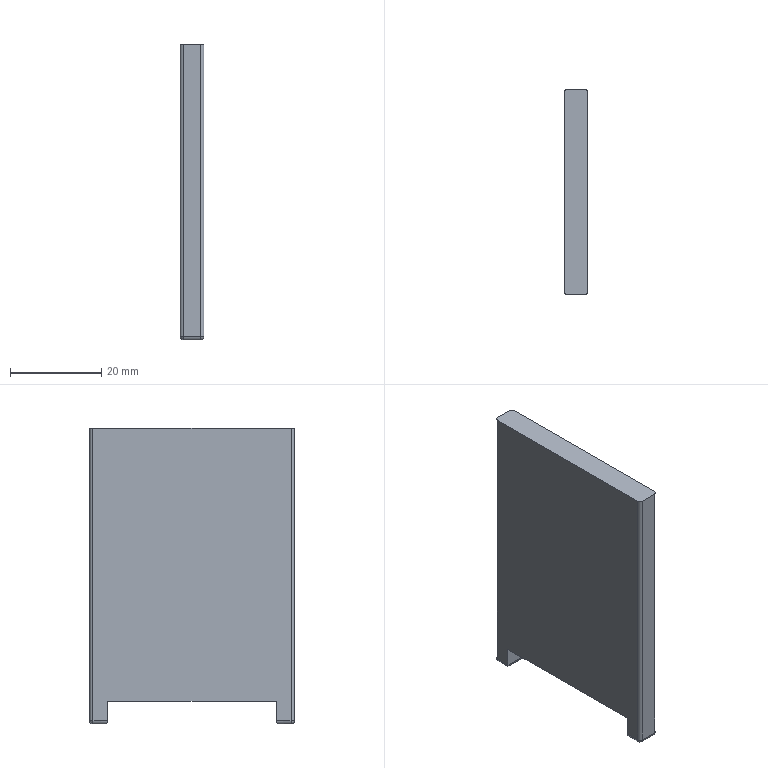Part | Creo | features DATUM PLANE 3, CURVE 2, COORDINATE SYSTEM 1, CUT 1, PROTRUSION 1, ROUND 1 | 1 solid | 26 faces | box 5.25 x 45 x 65 mm | volume 14350 mm3 | cylinder 12 | plane 10 | sphere 4 | commonest cylinder face diameters 1.5 x12
STEP:
#1=CARTESIAN_POINT('',(0.,0.,0.));
#2=DIRECTION('',(0.,0.,1.));
#3=DIRECTION('',(1.,0.,0.));
#4=AXIS2_PLACEMENT_3D('',#1,#2,#3);
#5=CARTESIAN_POINT('',(1.875,-19.25,0.));
#6=VERTEX_POINT('',#5);
#7=CARTESIAN_POINT('',(1.875,-21.75,0.));
#8=VERTEX_POINT('',#7);
#9=CARTESIAN_POINT('',(1.875,-19.25,0.));
#10=DIRECTION('',(0.,-1.,0.));
#11=VECTOR('',#10,2.5);
#12=LINE('',#9,#11);
#13=EDGE_CURVE('',#6,#8,#12,.T.);
#14=ORIENTED_EDGE('',*,*,#13,.F.);
#15=CARTESIAN_POINT('',(-1.875,-19.25,0.));
#16=VERTEX_POINT('',#15);
#17=CARTESIAN_POINT('',(-1.875,-19.25,0.));
#18=DIRECTION('',(1.,0.,0.));
#19=VECTOR('',#18,3.75);
#20=LINE('',#17,#19);
#21=EDGE_CURVE('',#16,#6,#20,.T.);
#22=ORIENTED_EDGE('',*,*,#21,.F.);
#23=CARTESIAN_POINT('',(-1.875,-21.75,0.));
#24=VERTEX_POINT('',#23);
#25=CARTESIAN_POINT('',(-1.875,-21.75,0.));
#26=DIRECTION('',(0.,1.,0.));
#27=VECTOR('',#26,2.5);
#28=LINE('',#25,#27);
#29=EDGE_CURVE('',#24,#16,#28,.T.);
#30=ORIENTED_EDGE('',*,*,#29,.F.);
#31=CARTESIAN_POINT('',(1.875,-21.75,0.));
#32=DIRECTION('',(-1.,0.,0.));
#33=VECTOR('',#32,3.75);
#34=LINE('',#31,#33);
#35=EDGE_CURVE('',#8,#24,#34,.T.);
#36=ORIENTED_EDGE('',*,*,#35,.F.);
#37=EDGE_LOOP('',(#14,#22,#30,#36));
#38=FACE_OUTER_BOUND('',#37,.F.);
#39=CARTESIAN_POINT('',(0.,0.,0.));
#40=DIRECTION('',(0.,0.,1.));
#41=DIRECTION('',(1.,0.,0.));
#42=AXIS2_PLACEMENT_3D('',#39,#40,#41);
#43=PLANE('',#42);
#44=ADVANCED_FACE('',(#38),#43,.F.);
#45=CARTESIAN_POINT('',(-1.875,21.75,0.));
#46=VERTEX_POINT('',#45);
#47=CARTESIAN_POINT('',(1.875,21.75,0.));
#48=VERTEX_POINT('',#47);
#49=CARTESIAN_POINT('',(-1.875,21.75,0.));
#50=DIRECTION('',(1.,0.,0.));
#51=VECTOR('',#50,3.75);
#52=LINE('',#49,#51);
#53=EDGE_CURVE('',#46,#48,#52,.T.);
#54=ORIENTED_EDGE('',*,*,#53,.F.);
#55=CARTESIAN_POINT('',(-1.875,19.25,0.));
#56=VERTEX_POINT('',#55);
#57=CARTESIAN_POINT('',(-1.875,19.25,0.));
#58=DIRECTION('',(0.,1.,0.));
#59=VECTOR('',#58,2.5);
#60=LINE('',#57,#59);
#61=EDGE_CURVE('',#56,#46,#60,.T.);
#62=ORIENTED_EDGE('',*,*,#61,.F.);
#63=CARTESIAN_POINT('',(1.875,19.25,0.));
#64=VERTEX_POINT('',#63);
#65=CARTESIAN_POINT('',(1.875,19.25,0.));
#66=DIRECTION('',(-1.,0.,0.));
#67=VECTOR('',#66,3.75);
#68=LINE('',#65,#67);
#69=EDGE_CURVE('',#64,#56,#68,.T.);
#70=ORIENTED_EDGE('',*,*,#69,.F.);
#71=CARTESIAN_POINT('',(1.875,21.75,0.));
#72=DIRECTION('',(0.,-1.,0.));
#73=VECTOR('',#72,2.5);
#74=LINE('',#71,#73);
#75=EDGE_CURVE('',#48,#64,#74,.T.);
#76=ORIENTED_EDGE('',*,*,#75,.F.);
#77=EDGE_LOOP('',(#54,#62,#70,#76));
#78=FACE_OUTER_BOUND('',#77,.F.);
#79=CARTESIAN_POINT('',(0.,0.,0.));
#80=DIRECTION('',(0.,0.,1.));
#81=DIRECTION('',(1.,0.,0.));
#82=AXIS2_PLACEMENT_3D('',#79,#80,#81);
#83=PLANE('',#82);
#84=ADVANCED_FACE('',(#78),#83,.F.);
#85=CARTESIAN_POINT('',(2.625,-18.5,0.75));
#86=VERTEX_POINT('',#85);
#87=CARTESIAN_POINT('',(2.625,-21.75,0.75));
#88=VERTEX_POINT('',#87);
#89=CARTESIAN_POINT('',(2.625,-18.5,0.75));
#90=DIRECTION('',(0.,-1.,0.));
#91=VECTOR('',#90,3.25);
#92=LINE('',#89,#91);
#93=EDGE_CURVE('',#86,#88,#92,.T.);
#94=ORIENTED_EDGE('',*,*,#93,.F.);
#95=CARTESIAN_POINT('',(2.625,-18.5,0.75));
#96=CARTESIAN_POINT('',(2.625,-18.5,0.6758));
#97=CARTESIAN_POINT('',(2.603,-18.522,0.5347));
#98=CARTESIAN_POINT('',(2.524,-18.601,0.3606));
#99=CARTESIAN_POINT('',(2.418,-18.707,0.2234));
#100=CARTESIAN_POINT('',(2.292,-18.833,0.1204));
#101=CARTESIAN_POINT('',(2.156,-18.969,0.04927));
#102=CARTESIAN_POINT('',(2.014,-19.111,0.008391));
#103=CARTESIAN_POINT('',(1.921,-19.204,0.));
#104=CARTESIAN_POINT('',(1.875,-19.25,0.));
#105=B_SPLINE_CURVE_WITH_KNOTS('',3,(#95,#96,#97,#98,#99,#100,#101,#102,#103,#104),.UNSPECIFIED.,.F.,.F.,(4,1,1,1,1,1,1,4),(0.,0.1429,0.2857,0.4286,0.5714,0.7143,0.8571,1.),.UNSPECIFIED.);
#106=EDGE_CURVE('',#86,#6,#105,.T.);
#107=ORIENTED_EDGE('',*,*,#106,.T.);
#108=ORIENTED_EDGE('',*,*,#13,.T.);
#109=CARTESIAN_POINT('',(1.875,-21.75,0.75));
#110=DIRECTION('',(0.,-1.,0.));
#111=DIRECTION('',(0.,0.,-1.));
#112=AXIS2_PLACEMENT_3D('',#109,#110,#111);
#113=CIRCLE('',#112,0.75);
#114=EDGE_CURVE('',#8,#88,#113,.T.);
#115=ORIENTED_EDGE('',*,*,#114,.T.);
#116=EDGE_LOOP('',(#94,#107,#108,#115));
#117=FACE_OUTER_BOUND('',#116,.F.);
#118=CARTESIAN_POINT('',(1.875,81.162,0.75));
#119=DIRECTION('',(0.,-1.,0.));
#120=DIRECTION('',(0.,0.,-1.));
#121=AXIS2_PLACEMENT_3D('',#118,#119,#120);
#122=CYLINDRICAL_SURFACE('',#121,0.75);
#123=ADVANCED_FACE('',(#117),#122,.T.);
#124=ORIENTED_EDGE('',*,*,#93,.T.);
#125=CARTESIAN_POINT('',(2.625,-21.75,65.));
#126=VERTEX_POINT('',#125);
#127=CARTESIAN_POINT('',(2.625,-21.75,65.));
#128=DIRECTION('',(0.,0.,-1.));
#129=VECTOR('',#128,64.25);
#130=LINE('',#127,#129);
#131=EDGE_CURVE('',#126,#88,#130,.T.);
#132=ORIENTED_EDGE('',*,*,#131,.F.);
#133=CARTESIAN_POINT('',(2.625,21.75,65.));
#134=VERTEX_POINT('',#133);
#135=CARTESIAN_POINT('',(2.625,-21.75,65.));
#136=DIRECTION('',(0.,1.,0.));
#137=VECTOR('',#136,43.5);
#138=LINE('',#135,#137);
#139=EDGE_CURVE('',#126,#134,#138,.T.);
#140=ORIENTED_EDGE('',*,*,#139,.T.);
#141=CARTESIAN_POINT('',(2.625,21.75,0.75));
#142=VERTEX_POINT('',#141);
#143=CARTESIAN_POINT('',(2.625,21.75,65.));
#144=DIRECTION('',(0.,0.,-1.));
#145=VECTOR('',#144,64.25);
#146=LINE('',#143,#145);
#147=EDGE_CURVE('',#134,#142,#146,.T.);
#148=ORIENTED_EDGE('',*,*,#147,.T.);
#149=CARTESIAN_POINT('',(2.625,18.5,0.75));
#150=VERTEX_POINT('',#149);
#151=CARTESIAN_POINT('',(2.625,21.75,0.75));
#152=DIRECTION('',(0.,-1.,0.));
#153=VECTOR('',#152,3.25);
#154=LINE('',#151,#153);
#155=EDGE_CURVE('',#142,#150,#154,.T.);
#156=ORIENTED_EDGE('',*,*,#155,.T.);
#157=CARTESIAN_POINT('',(2.625,18.5,5.));
#158=VERTEX_POINT('',#157);
#159=CARTESIAN_POINT('',(2.625,18.5,0.75));
#160=DIRECTION('',(0.,0.,1.));
#161=VECTOR('',#160,4.25);
#162=LINE('',#159,#161);
#163=EDGE_CURVE('',#150,#158,#162,.T.);
#164=ORIENTED_EDGE('',*,*,#163,.T.);
#165=CARTESIAN_POINT('',(2.625,-18.5,5.));
#166=VERTEX_POINT('',#165);
#167=CARTESIAN_POINT('',(2.625,18.5,5.));
#168=DIRECTION('',(0.,-1.,0.));
#169=VECTOR('',#168,37.);
#170=LINE('',#167,#169);
#171=EDGE_CURVE('',#158,#166,#170,.T.);
#172=ORIENTED_EDGE('',*,*,#171,.T.);
#173=CARTESIAN_POINT('',(2.625,-18.5,0.75));
#174=DIRECTION('',(0.,0.,1.));
#175=VECTOR('',#174,4.25);
#176=LINE('',#173,#175);
#177=EDGE_CURVE('',#86,#166,#176,.T.);
#178=ORIENTED_EDGE('',*,*,#177,.F.);
#179=EDGE_LOOP('',(#124,#132,#140,#148,#156,#164,#172,#178));
#180=FACE_OUTER_BOUND('',#179,.F.);
#181=CARTESIAN_POINT('',(2.625,-22.5,0.));
#182=DIRECTION('',(1.,0.,0.));
#183=DIRECTION('',(0.,1.,0.));
#184=AXIS2_PLACEMENT_3D('',#181,#182,#183);
#185=PLANE('',#184);
#186=ADVANCED_FACE('',(#180),#185,.T.);
#187=CARTESIAN_POINT('',(1.875,-22.5,65.));
#188=VERTEX_POINT('',#187);
#189=CARTESIAN_POINT('',(1.875,-21.75,65.));
#190=DIRECTION('',(0.,0.,1.));
#191=DIRECTION('',(0.,-1.,0.));
#192=AXIS2_PLACEMENT_3D('',#189,#190,#191);
#193=CIRCLE('',#192,0.75);
#194=EDGE_CURVE('',#188,#126,#193,.T.);
#195=ORIENTED_EDGE('',*,*,#194,.T.);
#196=ORIENTED_EDGE('',*,*,#131,.T.);
#197=CARTESIAN_POINT('',(1.875,-22.5,0.75));
#198=VERTEX_POINT('',#197);
#199=CARTESIAN_POINT('',(1.875,-21.75,0.75));
#200=DIRECTION('',(0.,0.,-1.));
#201=DIRECTION('',(1.,0.,0.));
#202=AXIS2_PLACEMENT_3D('',#199,#200,#201);
#203=CIRCLE('',#202,0.75);
#204=EDGE_CURVE('',#88,#198,#203,.T.);
#205=ORIENTED_EDGE('',*,*,#204,.T.);
#206=CARTESIAN_POINT('',(1.875,-22.5,65.));
#207=DIRECTION('',(0.,0.,-1.));
#208=VECTOR('',#207,64.25);
#209=LINE('',#206,#208);
#210=EDGE_CURVE('',#188,#198,#209,.T.);
#211=ORIENTED_EDGE('',*,*,#210,.F.);
#212=EDGE_LOOP('',(#195,#196,#205,#211));
#213=FACE_OUTER_BOUND('',#212,.F.);
#214=CARTESIAN_POINT('',(1.875,-21.75,149.734));
#215=DIRECTION('',(0.,0.,-1.));
#216=DIRECTION('',(1.,0.,0.));
#217=AXIS2_PLACEMENT_3D('',#214,#215,#216);
#218=CYLINDRICAL_SURFACE('',#217,0.75);
#219=ADVANCED_FACE('',(#213),#218,.T.);
#220=CARTESIAN_POINT('',(-2.625,-21.75,65.));
#221=VERTEX_POINT('',#220);
#222=CARTESIAN_POINT('',(-1.875,-22.5,65.));
#223=VERTEX_POINT('',#222);
#224=CARTESIAN_POINT('',(-1.875,-21.75,65.));
#225=DIRECTION('',(0.,0.,1.));
#226=DIRECTION('',(-1.,0.,0.));
#227=AXIS2_PLACEMENT_3D('',#224,#225,#226);
#228=CIRCLE('',#227,0.75);
#229=EDGE_CURVE('',#221,#223,#228,.T.);
#230=ORIENTED_EDGE('',*,*,#229,.F.);
#231=CARTESIAN_POINT('',(-2.625,21.75,65.));
#232=VERTEX_POINT('',#231);
#233=CARTESIAN_POINT('',(-2.625,21.75,65.));
#234=DIRECTION('',(0.,-1.,0.));
#235=VECTOR('',#234,43.5);
#236=LINE('',#233,#235);
#237=EDGE_CURVE('',#232,#221,#236,.T.);
#238=ORIENTED_EDGE('',*,*,#237,.F.);
#239=CARTESIAN_POINT('',(-1.875,22.5,65.));
#240=VERTEX_POINT('',#239);
#241=CARTESIAN_POINT('',(-1.875,21.75,65.));
#242=DIRECTION('',(0.,0.,1.));
#243=DIRECTION('',(0.,1.,0.));
#244=AXIS2_PLACEMENT_3D('',#241,#242,#243);
#245=CIRCLE('',#244,0.75);
#246=EDGE_CURVE('',#240,#232,#245,.T.);
#247=ORIENTED_EDGE('',*,*,#246,.F.);
#248=CARTESIAN_POINT('',(1.875,22.5,65.));
#249=VERTEX_POINT('',#248);
#250=CARTESIAN_POINT('',(1.875,22.5,65.));
#251=DIRECTION('',(-1.,0.,0.));
#252=VECTOR('',#251,3.75);
#253=LINE('',#250,#252);
#254=EDGE_CURVE('',#249,#240,#253,.T.);
#255=ORIENTED_EDGE('',*,*,#254,.F.);
#256=CARTESIAN_POINT('',(1.875,21.75,65.));
#257=DIRECTION('',(0.,0.,1.));
#258=DIRECTION('',(1.,0.,0.));
#259=AXIS2_PLACEMENT_3D('',#256,#257,#258);
#260=CIRCLE('',#259,0.75);
#261=EDGE_CURVE('',#134,#249,#260,.T.);
#262=ORIENTED_EDGE('',*,*,#261,.F.);
#263=ORIENTED_EDGE('',*,*,#139,.F.);
#264=ORIENTED_EDGE('',*,*,#194,.F.);
#265=CARTESIAN_POINT('',(-1.875,-22.5,65.));
#266=DIRECTION('',(1.,0.,0.));
#267=VECTOR('',#266,3.75);
#268=LINE('',#265,#267);
#269=EDGE_CURVE('',#223,#188,#268,.T.);
#270=ORIENTED_EDGE('',*,*,#269,.F.);
#271=EDGE_LOOP('',(#230,#238,#247,#255,#262,#263,#264,#270));
#272=FACE_OUTER_BOUND('',#271,.F.);
#273=CARTESIAN_POINT('',(0.,0.,65.));
#274=DIRECTION('',(0.,0.,1.));
#275=DIRECTION('',(1.,0.,0.));
#276=AXIS2_PLACEMENT_3D('',#273,#274,#275);
#277=PLANE('',#276);
#278=ADVANCED_FACE('',(#272),#277,.T.);
#279=ORIENTED_EDGE('',*,*,#229,.T.);
#280=CARTESIAN_POINT('',(-1.875,-22.5,0.75));
#281=VERTEX_POINT('',#280);
#282=CARTESIAN_POINT('',(-1.875,-22.5,65.));
#283=DIRECTION('',(0.,0.,-1.));
#284=VECTOR('',#283,64.25);
#285=LINE('',#282,#284);
#286=EDGE_CURVE('',#223,#281,#285,.T.);
#287=ORIENTED_EDGE('',*,*,#286,.T.);
#288=CARTESIAN_POINT('',(-2.625,-21.75,0.75));
#289=VERTEX_POINT('',#288);
#290=CARTESIAN_POINT('',(-1.875,-21.75,0.75));
#291=DIRECTION('',(0.,0.,-1.));
#292=DIRECTION('',(0.,-1.,0.));
#293=AXIS2_PLACEMENT_3D('',#290,#291,#292);
#294=CIRCLE('',#293,0.75);
#295=EDGE_CURVE('',#281,#289,#294,.T.);
#296=ORIENTED_EDGE('',*,*,#295,.T.);
#297=CARTESIAN_POINT('',(-2.625,-21.75,65.));
#298=DIRECTION('',(0.,0.,-1.));
#299=VECTOR('',#298,64.25);
#300=LINE('',#297,#299);
#301=EDGE_CURVE('',#221,#289,#300,.T.);
#302=ORIENTED_EDGE('',*,*,#301,.F.);
#303=EDGE_LOOP('',(#279,#287,#296,#302));
#304=FACE_OUTER_BOUND('',#303,.F.);
#305=CARTESIAN_POINT('',(-1.875,-21.75,149.734));
#306=DIRECTION('',(0.,0.,-1.));
#307=DIRECTION('',(0.,-1.,0.));
#308=AXIS2_PLACEMENT_3D('',#305,#306,#307);
#309=CYLINDRICAL_SURFACE('',#308,0.75);
#310=ADVANCED_FACE('',(#304),#309,.T.);
#311=ORIENTED_EDGE('',*,*,#286,.F.);
#312=ORIENTED_EDGE('',*,*,#269,.T.);
#313=ORIENTED_EDGE('',*,*,#210,.T.);
#314=CARTESIAN_POINT('',(1.875,-22.5,0.75));
#315=DIRECTION('',(-1.,0.,0.));
#316=VECTOR('',#315,3.75);
#317=LINE('',#314,#316);
#318=EDGE_CURVE('',#198,#281,#317,.T.);
#319=ORIENTED_EDGE('',*,*,#318,.T.);
#320=EDGE_LOOP('',(#311,#312,#313,#319));
#321=FACE_OUTER_BOUND('',#320,.F.);
#322=CARTESIAN_POINT('',(-2.625,-22.5,0.));
#323=DIRECTION('',(0.,-1.,0.));
#324=DIRECTION('',(1.,0.,0.));
#325=AXIS2_PLACEMENT_3D('',#322,#323,#324);
#326=PLANE('',#325);
#327=ADVANCED_FACE('',(#321),#326,.T.);
#328=ORIENTED_EDGE('',*,*,#318,.F.);
#329=CARTESIAN_POINT('',(1.875,-21.75,0.75));
#330=DIRECTION('',(1.,0.,0.));
#331=DIRECTION('',(0.,-1.,0.));
#332=AXIS2_PLACEMENT_3D('',#329,#330,#331);
#333=CIRCLE('',#332,0.75);
#334=EDGE_CURVE('',#198,#8,#333,.T.);
#335=ORIENTED_EDGE('',*,*,#334,.T.);
#336=ORIENTED_EDGE('',*,*,#35,.T.);
#337=CARTESIAN_POINT('',(-1.875,-21.75,0.75));
#338=DIRECTION('',(-1.,0.,0.));
#339=DIRECTION('',(0.,0.,-1.));
#340=AXIS2_PLACEMENT_3D('',#337,#338,#339);
#341=CIRCLE('',#340,0.75);
#342=EDGE_CURVE('',#24,#281,#341,.T.);
#343=ORIENTED_EDGE('',*,*,#342,.T.);
#344=EDGE_LOOP('',(#328,#335,#336,#343));
#345=FACE_OUTER_BOUND('',#344,.F.);
#346=CARTESIAN_POINT('',(9.469,-21.75,0.75));
#347=DIRECTION('',(-1.,0.,0.));
#348=DIRECTION('',(0.,0.,-1.));
#349=AXIS2_PLACEMENT_3D('',#346,#347,#348);
#350=CYLINDRICAL_SURFACE('',#349,0.75);
#351=ADVANCED_FACE('',(#345),#350,.T.);
#352=ORIENTED_EDGE('',*,*,#204,.F.);
#353=ORIENTED_EDGE('',*,*,#114,.F.);
#354=ORIENTED_EDGE('',*,*,#334,.F.);
#355=EDGE_LOOP('',(#352,#353,#354));
#356=FACE_OUTER_BOUND('',#355,.F.);
#357=CARTESIAN_POINT('',(1.875,-21.75,0.75));
#358=DIRECTION('',(0.,-0.7071,0.7071));
#359=DIRECTION('',(0.,-0.7071,-0.7071));
#360=AXIS2_PLACEMENT_3D('',#357,#358,#359);
#361=SPHERICAL_SURFACE('',#360,0.75);
#362=ADVANCED_FACE('',(#356),#361,.T.);
#363=ORIENTED_EDGE('',*,*,#342,.F.);
#364=CARTESIAN_POINT('',(-1.875,-21.75,0.75));
#365=DIRECTION('',(0.,-1.,0.));
#366=DIRECTION('',(-1.,0.,0.));
#367=AXIS2_PLACEMENT_3D('',#364,#365,#366);
#368=CIRCLE('',#367,0.75);
#369=EDGE_CURVE('',#289,#24,#368,.T.);
#370=ORIENTED_EDGE('',*,*,#369,.F.);
#371=ORIENTED_EDGE('',*,*,#295,.F.);
#372=EDGE_LOOP('',(#363,#370,#371));
#373=FACE_OUTER_BOUND('',#372,.F.);
#374=CARTESIAN_POINT('',(-1.875,-21.75,0.75));
#375=DIRECTION('',(0.7071,-0.7071,0.));
#376=DIRECTION('',(-0.7071,-0.7071,0.));
#377=AXIS2_PLACEMENT_3D('',#374,#375,#376);
#378=SPHERICAL_SURFACE('',#377,0.75);
#379=ADVANCED_FACE('',(#373),#378,.T.);
#380=CARTESIAN_POINT('',(-2.625,-18.5,0.75));
#381=VERTEX_POINT('',#380);
#382=CARTESIAN_POINT('',(-2.625,-21.75,0.75));
#383=DIRECTION('',(0.,1.,0.));
#384=VECTOR('',#383,3.25);
#385=LINE('',#382,#384);
#386=EDGE_CURVE('',#289,#381,#385,.T.);
#387=ORIENTED_EDGE('',*,*,#386,.F.);
#388=ORIENTED_EDGE('',*,*,#369,.T.);
#389=ORIENTED_EDGE('',*,*,#29,.T.);
#390=CARTESIAN_POINT('',(-2.625,-18.5,0.75));
#391=CARTESIAN_POINT('',(-2.625,-18.5,0.6758));
#392=CARTESIAN_POINT('',(-2.603,-18.522,0.5347));
#393=CARTESIAN_POINT('',(-2.524,-18.601,0.3606));
#394=CARTESIAN_POINT('',(-2.418,-18.707,0.2234));
#395=CARTESIAN_POINT('',(-2.292,-18.833,0.1204));
#396=CARTESIAN_POINT('',(-2.156,-18.969,0.04927));
#397=CARTESIAN_POINT('',(-2.014,-19.111,0.008391));
#398=CARTESIAN_POINT('',(-1.921,-19.204,0.));
#399=CARTESIAN_POINT('',(-1.875,-19.25,0.));
#400=B_SPLINE_CURVE_WITH_KNOTS('',3,(#390,#391,#392,#393,#394,#395,#396,#397,#398,#399),.UNSPECIFIED.,.F.,.F.,(4,1,1,1,1,1,1,4),(0.,0.1429,0.2857,0.4286,0.5714,0.7143,0.8571,1.),.UNSPECIFIED.);
#401=EDGE_CURVE('',#381,#16,#400,.T.);
#402=ORIENTED_EDGE('',*,*,#401,.F.);
#403=EDGE_LOOP('',(#387,#388,#389,#402));
#404=FACE_OUTER_BOUND('',#403,.F.);
#405=CARTESIAN_POINT('',(-1.875,-81.162,0.75));
#406=DIRECTION('',(0.,1.,0.));
#407=DIRECTION('',(0.,0.,-1.));
#408=AXIS2_PLACEMENT_3D('',#405,#406,#407);
#409=CYLINDRICAL_SURFACE('',#408,0.75);
#410=ADVANCED_FACE('',(#404),#409,.T.);
#411=ORIENTED_EDGE('',*,*,#386,.T.);
#412=CARTESIAN_POINT('',(-2.625,-18.5,5.));
#413=VERTEX_POINT('',#412);
#414=CARTESIAN_POINT('',(-2.625,-18.5,0.75));
#415=DIRECTION('',(0.,0.,1.));
#416=VECTOR('',#415,4.25);
#417=LINE('',#414,#416);
#418=EDGE_CURVE('',#381,#413,#417,.T.);
#419=ORIENTED_EDGE('',*,*,#418,.T.);
#420=CARTESIAN_POINT('',(-2.625,18.5,5.));
#421=VERTEX_POINT('',#420);
#422=CARTESIAN_POINT('',(-2.625,18.5,5.));
#423=DIRECTION('',(0.,-1.,0.));
#424=VECTOR('',#423,37.);
#425=LINE('',#422,#424);
#426=EDGE_CURVE('',#421,#413,#425,.T.);
#427=ORIENTED_EDGE('',*,*,#426,.F.);
#428=CARTESIAN_POINT('',(-2.625,18.5,0.75));
#429=VERTEX_POINT('',#428);
#430=CARTESIAN_POINT('',(-2.625,18.5,0.75));
#431=DIRECTION('',(0.,0.,1.));
#432=VECTOR('',#431,4.25);
#433=LINE('',#430,#432);
#434=EDGE_CURVE('',#429,#421,#433,.T.);
#435=ORIENTED_EDGE('',*,*,#434,.F.);
#436=CARTESIAN_POINT('',(-2.625,21.75,0.75));
#437=VERTEX_POINT('',#436);
#438=CARTESIAN_POINT('',(-2.625,18.5,0.75));
#439=DIRECTION('',(0.,1.,0.));
#440=VECTOR('',#439,3.25);
#441=LINE('',#438,#440);
#442=EDGE_CURVE('',#429,#437,#441,.T.);
#443=ORIENTED_EDGE('',*,*,#442,.T.);
#444=CARTESIAN_POINT('',(-2.625,21.75,65.));
#445=DIRECTION('',(0.,0.,-1.));
#446=VECTOR('',#445,64.25);
#447=LINE('',#444,#446);
#448=EDGE_CURVE('',#232,#437,#447,.T.);
#449=ORIENTED_EDGE('',*,*,#448,.F.);
#450=ORIENTED_EDGE('',*,*,#237,.T.);
#451=ORIENTED_EDGE('',*,*,#301,.T.);
#452=EDGE_LOOP('',(#411,#419,#427,#435,#443,#449,#450,#451));
#453=FACE_OUTER_BOUND('',#452,.F.);
#454=CARTESIAN_POINT('',(-2.625,22.5,0.));
#455=DIRECTION('',(-1.,0.,0.));
#456=DIRECTION('',(0.,-1.,0.));
#457=AXIS2_PLACEMENT_3D('',#454,#455,#456);
#458=PLANE('',#457);
#459=ADVANCED_FACE('',(#453),#458,.T.);
#460=CARTESIAN_POINT('',(-2.625,-18.5,0.75));
#461=DIRECTION('',(1.,0.,0.));
#462=VECTOR('',#461,5.25);
#463=LINE('',#460,#462);
#464=EDGE_CURVE('',#381,#86,#463,.T.);
#465=ORIENTED_EDGE('',*,*,#464,.T.);
#466=ORIENTED_EDGE('',*,*,#177,.T.);
#467=CARTESIAN_POINT('',(2.625,-18.5,5.));
#468=DIRECTION('',(-1.,0.,0.));
#469=VECTOR('',#468,5.25);
#470=LINE('',#467,#469);
#471=EDGE_CURVE('',#166,#413,#470,.T.);
#472=ORIENTED_EDGE('',*,*,#471,.T.);
#473=ORIENTED_EDGE('',*,*,#418,.F.);
#474=EDGE_LOOP('',(#465,#466,#472,#473));
#475=FACE_OUTER_BOUND('',#474,.F.);
#476=CARTESIAN_POINT('',(2.625,-18.5,5.));
#477=DIRECTION('',(0.,-1.,0.));
#478=DIRECTION('',(0.,0.,-1.));
#479=AXIS2_PLACEMENT_3D('',#476,#477,#478);
#480=PLANE('',#479);
#481=ADVANCED_FACE('',(#475),#480,.F.);
#482=ORIENTED_EDGE('',*,*,#21,.T.);
#483=ORIENTED_EDGE('',*,*,#106,.F.);
#484=ORIENTED_EDGE('',*,*,#464,.F.);
#485=ORIENTED_EDGE('',*,*,#401,.T.);
#486=EDGE_LOOP('',(#482,#483,#484,#485));
#487=FACE_OUTER_BOUND('',#486,.F.);
#488=CARTESIAN_POINT('',(-9.469,-19.25,0.75));
#489=DIRECTION('',(1.,0.,0.));
#490=DIRECTION('',(0.,0.,-1.));
#491=AXIS2_PLACEMENT_3D('',#488,#489,#490);
#492=CYLINDRICAL_SURFACE('',#491,0.75);
#493=ADVANCED_FACE('',(#487),#492,.T.);
#494=ORIENTED_EDGE('',*,*,#171,.F.);
#495=CARTESIAN_POINT('',(2.625,18.5,5.));
#496=DIRECTION('',(-1.,0.,0.));
#497=VECTOR('',#496,5.25);
#498=LINE('',#495,#497);
#499=EDGE_CURVE('',#158,#421,#498,.T.);
#500=ORIENTED_EDGE('',*,*,#499,.T.);
#501=ORIENTED_EDGE('',*,*,#426,.T.);
#502=ORIENTED_EDGE('',*,*,#471,.F.);
#503=EDGE_LOOP('',(#494,#500,#501,#502));
#504=FACE_OUTER_BOUND('',#503,.F.);
#505=CARTESIAN_POINT('',(2.625,18.5,5.));
#506=DIRECTION('',(0.,0.,1.));
#507=DIRECTION('',(0.,-1.,0.));
#508=AXIS2_PLACEMENT_3D('',#505,#506,#507);
#509=PLANE('',#508);
#510=ADVANCED_FACE('',(#504),#509,.F.);
#511=CARTESIAN_POINT('',(2.625,18.5,0.75));
#512=DIRECTION('',(-1.,0.,0.));
#513=VECTOR('',#512,5.25);
#514=LINE('',#511,#513);
#515=EDGE_CURVE('',#150,#429,#514,.T.);
#516=ORIENTED_EDGE('',*,*,#515,.T.);
#517=ORIENTED_EDGE('',*,*,#434,.T.);
#518=ORIENTED_EDGE('',*,*,#499,.F.);
#519=ORIENTED_EDGE('',*,*,#163,.F.);
#520=EDGE_LOOP('',(#516,#517,#518,#519));
#521=FACE_OUTER_BOUND('',#520,.F.);
#522=CARTESIAN_POINT('',(2.625,18.5,0.));
#523=DIRECTION('',(0.,1.,0.));
#524=DIRECTION('',(0.,0.,1.));
#525=AXIS2_PLACEMENT_3D('',#522,#523,#524);
#526=PLANE('',#525);
#527=ADVANCED_FACE('',(#521),#526,.F.);
#528=ORIENTED_EDGE('',*,*,#515,.F.);
#529=CARTESIAN_POINT('',(2.625,18.5,0.75));
#530=CARTESIAN_POINT('',(2.625,18.5,0.6758));
#531=CARTESIAN_POINT('',(2.603,18.522,0.5347));
#532=CARTESIAN_POINT('',(2.524,18.601,0.3606));
#533=CARTESIAN_POINT('',(2.418,18.707,0.2234));
#534=CARTESIAN_POINT('',(2.292,18.833,0.1204));
#535=CARTESIAN_POINT('',(2.156,18.969,0.04927));
#536=CARTESIAN_POINT('',(2.014,19.111,0.008391));
#537=CARTESIAN_POINT('',(1.921,19.204,0.));
#538=CARTESIAN_POINT('',(1.875,19.25,0.));
#539=B_SPLINE_CURVE_WITH_KNOTS('',3,(#529,#530,#531,#532,#533,#534,#535,#536,#537,#538),.UNSPECIFIED.,.F.,.F.,(4,1,1,1,1,1,1,4),(0.,0.1429,0.2857,0.4286,0.5714,0.7143,0.8571,1.),.UNSPECIFIED.);
#540=EDGE_CURVE('',#150,#64,#539,.T.);
#541=ORIENTED_EDGE('',*,*,#540,.T.);
#542=ORIENTED_EDGE('',*,*,#69,.T.);
#543=CARTESIAN_POINT('',(-2.625,18.5,0.75));
#544=CARTESIAN_POINT('',(-2.625,18.5,0.6758));
#545=CARTESIAN_POINT('',(-2.603,18.522,0.5347));
#546=CARTESIAN_POINT('',(-2.524,18.601,0.3606));
#547=CARTESIAN_POINT('',(-2.418,18.707,0.2234));
#548=CARTESIAN_POINT('',(-2.292,18.833,0.1204));
#549=CARTESIAN_POINT('',(-2.156,18.969,0.04927));
#550=CARTESIAN_POINT('',(-2.014,19.111,0.008391));
#551=CARTESIAN_POINT('',(-1.921,19.204,0.));
#552=CARTESIAN_POINT('',(-1.875,19.25,0.));
#553=B_SPLINE_CURVE_WITH_KNOTS('',3,(#543,#544,#545,#546,#547,#548,#549,#550,#551,#552),.UNSPECIFIED.,.F.,.F.,(4,1,1,1,1,1,1,4),(0.,0.1429,0.2857,0.4286,0.5714,0.7143,0.8571,1.),.UNSPECIFIED.);
#554=EDGE_CURVE('',#429,#56,#553,.T.);
#555=ORIENTED_EDGE('',*,*,#554,.F.);
#556=EDGE_LOOP('',(#528,#541,#542,#555));
#557=FACE_OUTER_BOUND('',#556,.F.);
#558=CARTESIAN_POINT('',(9.469,19.25,0.75));
#559=DIRECTION('',(-1.,0.,0.));
#560=DIRECTION('',(0.,0.,-1.));
#561=AXIS2_PLACEMENT_3D('',#558,#559,#560);
#562=CYLINDRICAL_SURFACE('',#561,0.75);
#563=ADVANCED_FACE('',(#557),#562,.T.);
#564=ORIENTED_EDGE('',*,*,#155,.F.);
#565=CARTESIAN_POINT('',(1.875,21.75,0.75));
#566=DIRECTION('',(0.,1.,0.));
#567=DIRECTION('',(1.,0.,0.));
#568=AXIS2_PLACEMENT_3D('',#565,#566,#567);
#569=CIRCLE('',#568,0.75);
#570=EDGE_CURVE('',#142,#48,#569,.T.);
#571=ORIENTED_EDGE('',*,*,#570,.T.);
#572=ORIENTED_EDGE('',*,*,#75,.T.);
#573=ORIENTED_EDGE('',*,*,#540,.F.);
#574=EDGE_LOOP('',(#564,#571,#572,#573));
#575=FACE_OUTER_BOUND('',#574,.F.);
#576=CARTESIAN_POINT('',(1.875,81.162,0.75));
#577=DIRECTION('',(0.,-1.,0.));
#578=DIRECTION('',(0.,0.,-1.));
#579=AXIS2_PLACEMENT_3D('',#576,#577,#578);
#580=CYLINDRICAL_SURFACE('',#579,0.75);
#581=ADVANCED_FACE('',(#575),#580,.T.);
#582=ORIENTED_EDGE('',*,*,#570,.F.);
#583=CARTESIAN_POINT('',(1.875,22.5,0.75));
#584=VERTEX_POINT('',#583);
#585=CARTESIAN_POINT('',(1.875,21.75,0.75));
#586=DIRECTION('',(0.,0.,-1.));
#587=DIRECTION('',(0.,1.,0.));
#588=AXIS2_PLACEMENT_3D('',#585,#586,#587);
#589=CIRCLE('',#588,0.75);
#590=EDGE_CURVE('',#584,#142,#589,.T.);
#591=ORIENTED_EDGE('',*,*,#590,.F.);
#592=CARTESIAN_POINT('',(1.875,21.75,0.75));
#593=DIRECTION('',(1.,0.,0.));
#594=DIRECTION('',(0.,0.,-1.));
#595=AXIS2_PLACEMENT_3D('',#592,#593,#594);
#596=CIRCLE('',#595,0.75);
#597=EDGE_CURVE('',#48,#584,#596,.T.);
#598=ORIENTED_EDGE('',*,*,#597,.F.);
#599=EDGE_LOOP('',(#582,#591,#598));
#600=FACE_OUTER_BOUND('',#599,.F.);
#601=CARTESIAN_POINT('',(1.875,21.75,0.75));
#602=DIRECTION('',(-0.7071,0.7071,0.));
#603=DIRECTION('',(0.7071,0.7071,0.));
#604=AXIS2_PLACEMENT_3D('',#601,#602,#603);
#605=SPHERICAL_SURFACE('',#604,0.75);
#606=ADVANCED_FACE('',(#600),#605,.T.);
#607=ORIENTED_EDGE('',*,*,#261,.T.);
#608=CARTESIAN_POINT('',(1.875,22.5,65.));
#609=DIRECTION('',(0.,0.,-1.));
#610=VECTOR('',#609,64.25);
#611=LINE('',#608,#610);
#612=EDGE_CURVE('',#249,#584,#611,.T.);
#613=ORIENTED_EDGE('',*,*,#612,.T.);
#614=ORIENTED_EDGE('',*,*,#590,.T.);
#615=ORIENTED_EDGE('',*,*,#147,.F.);
#616=EDGE_LOOP('',(#607,#613,#614,#615));
#617=FACE_OUTER_BOUND('',#616,.F.);
#618=CARTESIAN_POINT('',(1.875,21.75,149.734));
#619=DIRECTION('',(0.,0.,-1.));
#620=DIRECTION('',(0.,1.,0.));
#621=AXIS2_PLACEMENT_3D('',#618,#619,#620);
#622=CYLINDRICAL_SURFACE('',#621,0.75);
#623=ADVANCED_FACE('',(#617),#622,.T.);
#624=ORIENTED_EDGE('',*,*,#612,.F.);
#625=ORIENTED_EDGE('',*,*,#254,.T.);
#626=CARTESIAN_POINT('',(-1.875,22.5,0.75));
#627=VERTEX_POINT('',#626);
#628=CARTESIAN_POINT('',(-1.875,22.5,65.));
#629=DIRECTION('',(0.,0.,-1.));
#630=VECTOR('',#629,64.25);
#631=LINE('',#628,#630);
#632=EDGE_CURVE('',#240,#627,#631,.T.);
#633=ORIENTED_EDGE('',*,*,#632,.T.);
#634=CARTESIAN_POINT('',(-1.875,22.5,0.75));
#635=DIRECTION('',(1.,0.,0.));
#636=VECTOR('',#635,3.75);
#637=LINE('',#634,#636);
#638=EDGE_CURVE('',#627,#584,#637,.T.);
#639=ORIENTED_EDGE('',*,*,#638,.T.);
#640=EDGE_LOOP('',(#624,#625,#633,#639));
#641=FACE_OUTER_BOUND('',#640,.F.);
#642=CARTESIAN_POINT('',(2.625,22.5,0.));
#643=DIRECTION('',(0.,1.,0.));
#644=DIRECTION('',(-1.,0.,0.));
#645=AXIS2_PLACEMENT_3D('',#642,#643,#644);
#646=PLANE('',#645);
#647=ADVANCED_FACE('',(#641),#646,.T.);
#648=ORIENTED_EDGE('',*,*,#246,.T.);
#649=ORIENTED_EDGE('',*,*,#448,.T.);
#650=CARTESIAN_POINT('',(-1.875,21.75,0.75));
#651=DIRECTION('',(0.,0.,-1.));
#652=DIRECTION('',(-1.,0.,0.));
#653=AXIS2_PLACEMENT_3D('',#650,#651,#652);
#654=CIRCLE('',#653,0.75);
#655=EDGE_CURVE('',#437,#627,#654,.T.);
#656=ORIENTED_EDGE('',*,*,#655,.T.);
#657=ORIENTED_EDGE('',*,*,#632,.F.);
#658=EDGE_LOOP('',(#648,#649,#656,#657));
#659=FACE_OUTER_BOUND('',#658,.F.);
#660=CARTESIAN_POINT('',(-1.875,21.75,149.734));
#661=DIRECTION('',(0.,0.,-1.));
#662=DIRECTION('',(-1.,0.,0.));
#663=AXIS2_PLACEMENT_3D('',#660,#661,#662);
#664=CYLINDRICAL_SURFACE('',#663,0.75);
#665=ADVANCED_FACE('',(#659),#664,.T.);
#666=ORIENTED_EDGE('',*,*,#655,.F.);
#667=CARTESIAN_POINT('',(-1.875,21.75,0.75));
#668=DIRECTION('',(0.,1.,0.));
#669=DIRECTION('',(0.,0.,-1.));
#670=AXIS2_PLACEMENT_3D('',#667,#668,#669);
#671=CIRCLE('',#670,0.75);
#672=EDGE_CURVE('',#46,#437,#671,.T.);
#673=ORIENTED_EDGE('',*,*,#672,.F.);
#674=CARTESIAN_POINT('',(-1.875,21.75,0.75));
#675=DIRECTION('',(-1.,0.,0.));
#676=DIRECTION('',(0.,1.,0.));
#677=AXIS2_PLACEMENT_3D('',#674,#675,#676);
#678=CIRCLE('',#677,0.75);
#679=EDGE_CURVE('',#627,#46,#678,.T.);
#680=ORIENTED_EDGE('',*,*,#679,.F.);
#681=EDGE_LOOP('',(#666,#673,#680));
#682=FACE_OUTER_BOUND('',#681,.F.);
#683=CARTESIAN_POINT('',(-1.875,21.75,0.75));
#684=DIRECTION('',(-0.7071,-0.7071,0.));
#685=DIRECTION('',(-0.7071,0.7071,0.));
#686=AXIS2_PLACEMENT_3D('',#683,#684,#685);
#687=SPHERICAL_SURFACE('',#686,0.75);
#688=ADVANCED_FACE('',(#682),#687,.T.);
#689=ORIENTED_EDGE('',*,*,#61,.T.);
#690=ORIENTED_EDGE('',*,*,#672,.T.);
#691=ORIENTED_EDGE('',*,*,#442,.F.);
#692=ORIENTED_EDGE('',*,*,#554,.T.);
#693=EDGE_LOOP('',(#689,#690,#691,#692));
#694=FACE_OUTER_BOUND('',#693,.F.);
#695=CARTESIAN_POINT('',(-1.875,-81.162,0.75));
#696=DIRECTION('',(0.,1.,0.));
#697=DIRECTION('',(0.,0.,-1.));
#698=AXIS2_PLACEMENT_3D('',#695,#696,#697);
#699=CYLINDRICAL_SURFACE('',#698,0.75);
#700=ADVANCED_FACE('',(#694),#699,.T.);
#701=ORIENTED_EDGE('',*,*,#53,.T.);
#702=ORIENTED_EDGE('',*,*,#597,.T.);
#703=ORIENTED_EDGE('',*,*,#638,.F.);
#704=ORIENTED_EDGE('',*,*,#679,.T.);
#705=EDGE_LOOP('',(#701,#702,#703,#704));
#706=FACE_OUTER_BOUND('',#705,.F.);
#707=CARTESIAN_POINT('',(-9.469,21.75,0.75));
#708=DIRECTION('',(1.,0.,0.));
#709=DIRECTION('',(0.,0.,-1.));
#710=AXIS2_PLACEMENT_3D('',#707,#708,#709);
#711=CYLINDRICAL_SURFACE('',#710,0.75);
#712=ADVANCED_FACE('',(#706),#711,.T.);
#713=CLOSED_SHELL('',(#44,#84,#123,#186,#219,#278,#310,#327,#351,#362,#379,#410,#459,#481,#493,#510,#527,#563,#581,#606,#623,#647,#665,#688,#700,#712));
#714=MANIFOLD_SOLID_BREP('',#713);
#715=(LENGTH_UNIT()NAMED_UNIT(*)SI_UNIT(.MILLI.,.METRE.));
#716=UNCERTAINTY_MEASURE_WITH_UNIT(LENGTH_MEASURE(0.007923),#715,'','');
#717=(NAMED_UNIT(*)PLANE_ANGLE_UNIT()SI_UNIT($,.RADIAN.));
#718=PLANE_ANGLE_MEASURE_WITH_UNIT(PLANE_ANGLE_MEASURE(0.01745),#717);
#719=(CONVERSION_BASED_UNIT('DEGREE',#718)NAMED_UNIT(*)PLANE_ANGLE_UNIT());
#720=(NAMED_UNIT(*)SI_UNIT($,.STERADIAN.)SOLID_ANGLE_UNIT());
#721=(GEOMETRIC_REPRESENTATION_CONTEXT(3)GLOBAL_UNCERTAINTY_ASSIGNED_CONTEXT((#716))GLOBAL_UNIT_ASSIGNED_CONTEXT((#715,#719,#720))REPRESENTATION_CONTEXT('',''));
#722=ADVANCED_BREP_SHAPE_REPRESENTATION('',(#4,#714),#721);